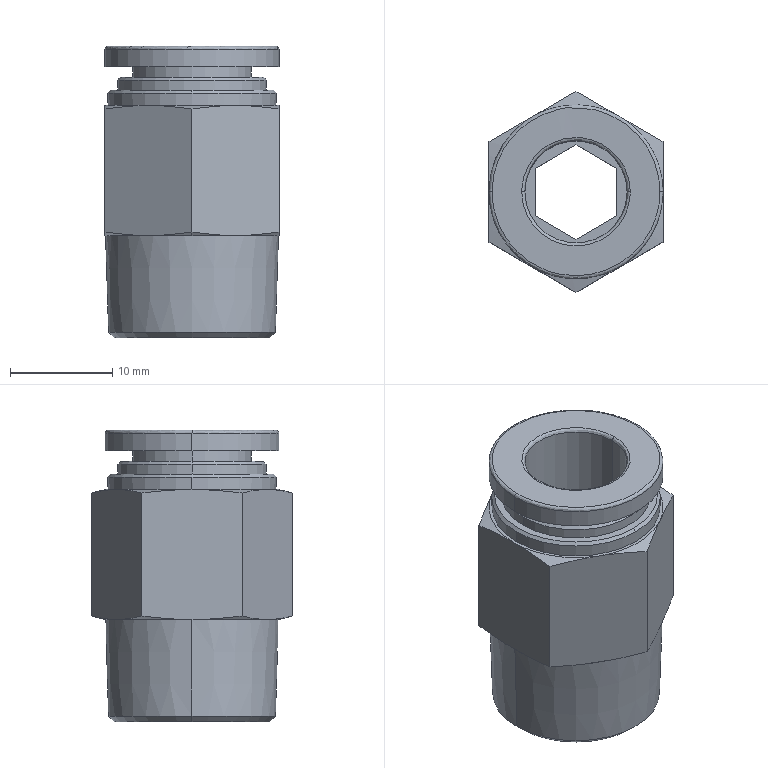Part | STEP file | KZB175-10-03-175 | 1 solid | 60 faces | box 17 x 19.63 x 28.5 mm | volume 4009 mm3 | cone 25 | plane 21 | cylinder 10 | spline 4 | commonest cylinder face diameters 10 x2 11.6 x2 12.2 x2 14.55 x2 17 x2